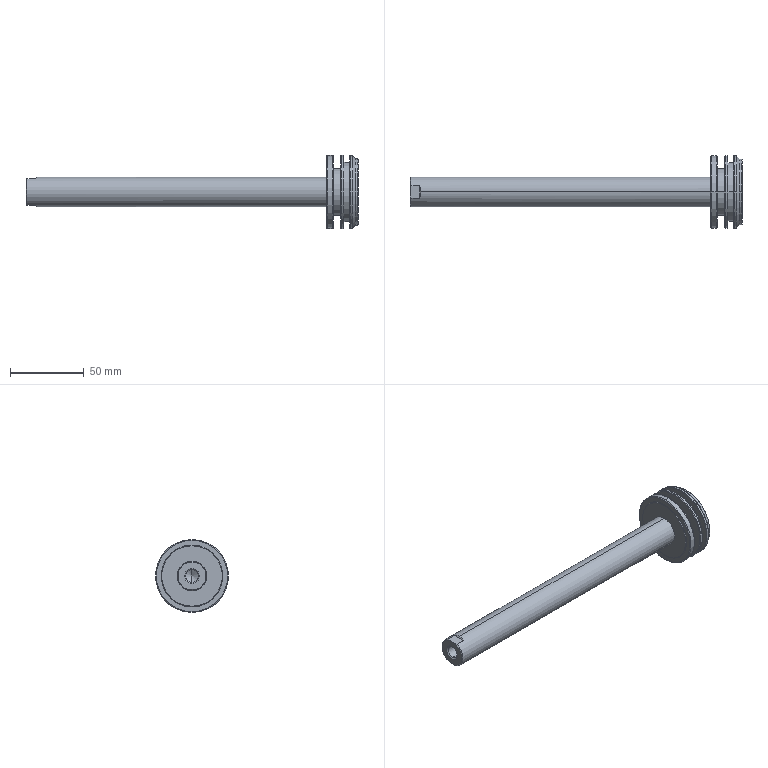Part | STEP file | TC_L_50x175_175r | 1 solid | 52 faces | box 225 x 49.5 x 49.5 mm | volume 94503 mm3 | cylinder 16 | cone 12 | torus 12 | plane 12 | commonest cylinder face diameters 49.5 x6 8.376 x2 20 x2 31.8 x2 40 x2 45 x2